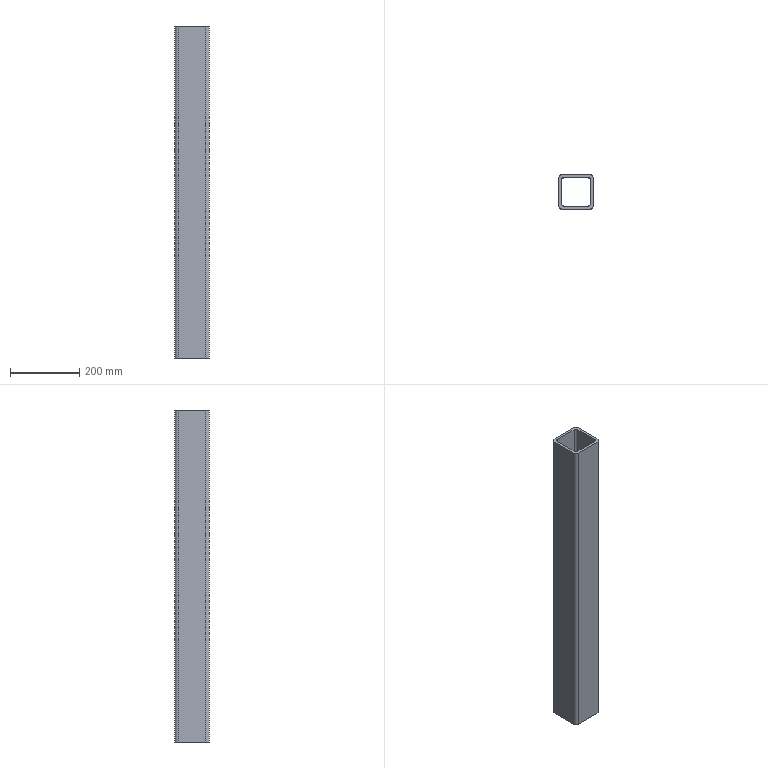Part | SolidWorks | features BaseBody 1 | 1 solid | 18 faces | box 100 x 100 x 960 mm | volume 2796573 mm3 | plane 10 | cylinder 8 | commonest cylinder face diameters 16 x4 20 x4
STEP:
#1=CARTESIAN_POINT('',(10.,96.35,960.));
#2=VERTEX_POINT('',#1);
#3=CARTESIAN_POINT('',(10.,96.35,0.));
#4=VERTEX_POINT('',#3);
#5=CARTESIAN_POINT('',(10.,96.35,960.));
#6=DIRECTION('',(0.,0.,-1.));
#7=VECTOR('',#6,1000.);
#8=LINE('',#5,#7);
#9=EDGE_CURVE('',#2,#4,#8,.T.);
#10=ORIENTED_EDGE('',*,*,#9,.F.);
#11=CARTESIAN_POINT('',(90.,96.35,960.));
#12=VERTEX_POINT('',#11);
#13=CARTESIAN_POINT('',(90.,96.35,960.));
#14=DIRECTION('',(-1.,0.,0.));
#15=VECTOR('',#14,1000.);
#16=LINE('',#13,#15);
#17=EDGE_CURVE('',#12,#2,#16,.T.);
#18=ORIENTED_EDGE('',*,*,#17,.F.);
#19=CARTESIAN_POINT('',(90.,96.35,0.));
#20=VERTEX_POINT('',#19);
#21=CARTESIAN_POINT('',(90.,96.35,960.));
#22=DIRECTION('',(0.,0.,1.));
#23=VECTOR('',#22,1000.);
#24=LINE('',#21,#23);
#25=EDGE_CURVE('',#20,#12,#24,.T.);
#26=ORIENTED_EDGE('',*,*,#25,.F.);
#27=CARTESIAN_POINT('',(90.,96.35,0.));
#28=DIRECTION('',(1.,0.,0.));
#29=VECTOR('',#28,1000.);
#30=LINE('',#27,#29);
#31=EDGE_CURVE('',#4,#20,#30,.T.);
#32=ORIENTED_EDGE('',*,*,#31,.F.);
#33=EDGE_LOOP('',(#10,#18,#26,#32));
#34=FACE_OUTER_BOUND('',#33,.T.);
#35=CARTESIAN_POINT('',(90.,96.35,960.));
#36=DIRECTION('',(0.,-1.,0.));
#37=DIRECTION('',(1.,0.,0.));
#38=AXIS2_PLACEMENT_3D('',#35,#36,#37);
#39=PLANE('',#38);
#40=ADVANCED_FACE('',(#34),#39,.F.);
#41=CARTESIAN_POINT('',(84.,4.35,0.));
#42=VERTEX_POINT('',#41);
#43=CARTESIAN_POINT('',(16.,4.35,0.));
#44=VERTEX_POINT('',#43);
#45=CARTESIAN_POINT('',(10.,4.35,0.));
#46=DIRECTION('',(-1.,0.,0.));
#47=VECTOR('',#46,1000.);
#48=LINE('',#45,#47);
#49=EDGE_CURVE('',#42,#44,#48,.T.);
#50=ORIENTED_EDGE('',*,*,#49,.F.);
#51=CARTESIAN_POINT('',(92.,12.35,0.));
#52=VERTEX_POINT('',#51);
#53=CARTESIAN_POINT('',(84.,12.35,0.));
#54=DIRECTION('',(0.,0.,-1.));
#55=DIRECTION('',(-1.,0.,0.));
#56=AXIS2_PLACEMENT_3D('',#53,#54,#55);
#57=CIRCLE('',#56,8.);
#58=EDGE_CURVE('',#52,#42,#57,.T.);
#59=ORIENTED_EDGE('',*,*,#58,.F.);
#60=CARTESIAN_POINT('',(92.,80.35,0.));
#61=VERTEX_POINT('',#60);
#62=CARTESIAN_POINT('',(92.,86.35,0.));
#63=DIRECTION('',(0.,-1.,0.));
#64=VECTOR('',#63,1000.);
#65=LINE('',#62,#64);
#66=EDGE_CURVE('',#61,#52,#65,.T.);
#67=ORIENTED_EDGE('',*,*,#66,.F.);
#68=CARTESIAN_POINT('',(84.,88.35,0.));
#69=VERTEX_POINT('',#68);
#70=CARTESIAN_POINT('',(84.,80.35,0.));
#71=DIRECTION('',(0.,0.,-1.));
#72=DIRECTION('',(-1.,0.,0.));
#73=AXIS2_PLACEMENT_3D('',#70,#71,#72);
#74=CIRCLE('',#73,8.);
#75=EDGE_CURVE('',#69,#61,#74,.T.);
#76=ORIENTED_EDGE('',*,*,#75,.F.);
#77=CARTESIAN_POINT('',(16.,88.35,0.));
#78=VERTEX_POINT('',#77);
#79=CARTESIAN_POINT('',(10.,88.35,0.));
#80=DIRECTION('',(1.,0.,0.));
#81=VECTOR('',#80,1000.);
#82=LINE('',#79,#81);
#83=EDGE_CURVE('',#78,#69,#82,.T.);
#84=ORIENTED_EDGE('',*,*,#83,.F.);
#85=CARTESIAN_POINT('',(8.,80.35,0.));
#86=VERTEX_POINT('',#85);
#87=CARTESIAN_POINT('',(16.,80.35,0.));
#88=DIRECTION('',(0.,0.,-1.));
#89=DIRECTION('',(-1.,0.,0.));
#90=AXIS2_PLACEMENT_3D('',#87,#88,#89);
#91=CIRCLE('',#90,8.);
#92=EDGE_CURVE('',#86,#78,#91,.T.);
#93=ORIENTED_EDGE('',*,*,#92,.F.);
#94=CARTESIAN_POINT('',(8.,12.35,0.));
#95=VERTEX_POINT('',#94);
#96=CARTESIAN_POINT('',(8.,86.35,0.));
#97=DIRECTION('',(0.,1.,0.));
#98=VECTOR('',#97,1000.);
#99=LINE('',#96,#98);
#100=EDGE_CURVE('',#95,#86,#99,.T.);
#101=ORIENTED_EDGE('',*,*,#100,.F.);
#102=CARTESIAN_POINT('',(16.,12.35,0.));
#103=DIRECTION('',(0.,0.,-1.));
#104=DIRECTION('',(-1.,0.,0.));
#105=AXIS2_PLACEMENT_3D('',#102,#103,#104);
#106=CIRCLE('',#105,8.);
#107=EDGE_CURVE('',#44,#95,#106,.T.);
#108=ORIENTED_EDGE('',*,*,#107,.F.);
#109=EDGE_LOOP('',(#50,#59,#67,#76,#84,#93,#101,#108));
#110=FACE_BOUND('',#109,.T.);
#111=CARTESIAN_POINT('',(100.,86.35,0.));
#112=VERTEX_POINT('',#111);
#113=CARTESIAN_POINT('',(90.,86.35,0.));
#114=DIRECTION('',(0.,0.,1.));
#115=DIRECTION('',(-1.,0.,0.));
#116=AXIS2_PLACEMENT_3D('',#113,#114,#115);
#117=CIRCLE('',#116,10.);
#118=EDGE_CURVE('',#112,#20,#117,.T.);
#119=ORIENTED_EDGE('',*,*,#118,.F.);
#120=CARTESIAN_POINT('',(100.,6.35,0.));
#121=VERTEX_POINT('',#120);
#122=CARTESIAN_POINT('',(100.,86.35,0.));
#123=DIRECTION('',(0.,1.,0.));
#124=VECTOR('',#123,1000.);
#125=LINE('',#122,#124);
#126=EDGE_CURVE('',#121,#112,#125,.T.);
#127=ORIENTED_EDGE('',*,*,#126,.F.);
#128=CARTESIAN_POINT('',(90.,-3.65,0.));
#129=VERTEX_POINT('',#128);
#130=CARTESIAN_POINT('',(90.,6.35,0.));
#131=DIRECTION('',(0.,0.,1.));
#132=DIRECTION('',(-1.,0.,0.));
#133=AXIS2_PLACEMENT_3D('',#130,#131,#132);
#134=CIRCLE('',#133,10.);
#135=EDGE_CURVE('',#129,#121,#134,.T.);
#136=ORIENTED_EDGE('',*,*,#135,.F.);
#137=CARTESIAN_POINT('',(10.,-3.65,0.));
#138=VERTEX_POINT('',#137);
#139=CARTESIAN_POINT('',(10.,-3.65,0.));
#140=DIRECTION('',(1.,0.,0.));
#141=VECTOR('',#140,1000.);
#142=LINE('',#139,#141);
#143=EDGE_CURVE('',#138,#129,#142,.T.);
#144=ORIENTED_EDGE('',*,*,#143,.F.);
#145=CARTESIAN_POINT('',(0.,6.35,0.));
#146=VERTEX_POINT('',#145);
#147=CARTESIAN_POINT('',(10.,6.35,0.));
#148=DIRECTION('',(0.,0.,1.));
#149=DIRECTION('',(-1.,0.,0.));
#150=AXIS2_PLACEMENT_3D('',#147,#148,#149);
#151=CIRCLE('',#150,10.);
#152=EDGE_CURVE('',#146,#138,#151,.T.);
#153=ORIENTED_EDGE('',*,*,#152,.F.);
#154=CARTESIAN_POINT('',(0.,86.35,0.));
#155=VERTEX_POINT('',#154);
#156=CARTESIAN_POINT('',(0.,86.35,0.));
#157=DIRECTION('',(0.,-1.,0.));
#158=VECTOR('',#157,1000.);
#159=LINE('',#156,#158);
#160=EDGE_CURVE('',#155,#146,#159,.T.);
#161=ORIENTED_EDGE('',*,*,#160,.F.);
#162=CARTESIAN_POINT('',(10.,86.35,0.));
#163=DIRECTION('',(0.,0.,1.));
#164=DIRECTION('',(-1.,0.,0.));
#165=AXIS2_PLACEMENT_3D('',#162,#163,#164);
#166=CIRCLE('',#165,10.);
#167=EDGE_CURVE('',#4,#155,#166,.T.);
#168=ORIENTED_EDGE('',*,*,#167,.F.);
#169=ORIENTED_EDGE('',*,*,#31,.T.);
#170=EDGE_LOOP('',(#119,#127,#136,#144,#153,#161,#168,#169));
#171=FACE_OUTER_BOUND('',#170,.T.);
#172=CARTESIAN_POINT('',(10.,86.35,0.));
#173=DIRECTION('',(0.,0.,1.));
#174=DIRECTION('',(1.,0.,0.));
#175=AXIS2_PLACEMENT_3D('',#172,#173,#174);
#176=PLANE('',#175);
#177=ADVANCED_FACE('',(#110,#171),#176,.F.);
#178=CARTESIAN_POINT('',(0.,86.35,960.));
#179=VERTEX_POINT('',#178);
#180=CARTESIAN_POINT('',(10.,86.35,960.));
#181=DIRECTION('',(0.,0.,-1.));
#182=DIRECTION('',(-1.,0.,0.));
#183=AXIS2_PLACEMENT_3D('',#180,#181,#182);
#184=CIRCLE('',#183,10.);
#185=EDGE_CURVE('',#179,#2,#184,.T.);
#186=ORIENTED_EDGE('',*,*,#185,.T.);
#187=ORIENTED_EDGE('',*,*,#9,.T.);
#188=ORIENTED_EDGE('',*,*,#167,.T.);
#189=CARTESIAN_POINT('',(0.,86.35,960.));
#190=DIRECTION('',(0.,0.,1.));
#191=VECTOR('',#190,1000.);
#192=LINE('',#189,#191);
#193=EDGE_CURVE('',#155,#179,#192,.T.);
#194=ORIENTED_EDGE('',*,*,#193,.T.);
#195=EDGE_LOOP('',(#186,#187,#188,#194));
#196=FACE_OUTER_BOUND('',#195,.T.);
#197=CARTESIAN_POINT('',(10.,86.35,960.));
#198=DIRECTION('',(0.,0.,-1.));
#199=DIRECTION('',(-1.,0.,0.));
#200=AXIS2_PLACEMENT_3D('',#197,#198,#199);
#201=CYLINDRICAL_SURFACE('',#200,10.);
#202=ADVANCED_FACE('',(#196),#201,.T.);
#203=CARTESIAN_POINT('',(92.,80.35,960.));
#204=VERTEX_POINT('',#203);
#205=CARTESIAN_POINT('',(92.,12.35,960.));
#206=VERTEX_POINT('',#205);
#207=CARTESIAN_POINT('',(92.,86.35,960.));
#208=DIRECTION('',(0.,-1.,0.));
#209=VECTOR('',#208,1000.);
#210=LINE('',#207,#209);
#211=EDGE_CURVE('',#204,#206,#210,.T.);
#212=ORIENTED_EDGE('',*,*,#211,.T.);
#213=CARTESIAN_POINT('',(84.,4.35,960.));
#214=VERTEX_POINT('',#213);
#215=CARTESIAN_POINT('',(84.,12.35,960.));
#216=DIRECTION('',(0.,0.,-1.));
#217=DIRECTION('',(-1.,0.,0.));
#218=AXIS2_PLACEMENT_3D('',#215,#216,#217);
#219=CIRCLE('',#218,8.);
#220=EDGE_CURVE('',#206,#214,#219,.T.);
#221=ORIENTED_EDGE('',*,*,#220,.T.);
#222=CARTESIAN_POINT('',(16.,4.35,960.));
#223=VERTEX_POINT('',#222);
#224=CARTESIAN_POINT('',(10.,4.35,960.));
#225=DIRECTION('',(-1.,0.,0.));
#226=VECTOR('',#225,1000.);
#227=LINE('',#224,#226);
#228=EDGE_CURVE('',#214,#223,#227,.T.);
#229=ORIENTED_EDGE('',*,*,#228,.T.);
#230=CARTESIAN_POINT('',(8.,12.35,960.));
#231=VERTEX_POINT('',#230);
#232=CARTESIAN_POINT('',(16.,12.35,960.));
#233=DIRECTION('',(0.,0.,-1.));
#234=DIRECTION('',(-1.,0.,0.));
#235=AXIS2_PLACEMENT_3D('',#232,#233,#234);
#236=CIRCLE('',#235,8.);
#237=EDGE_CURVE('',#223,#231,#236,.T.);
#238=ORIENTED_EDGE('',*,*,#237,.T.);
#239=CARTESIAN_POINT('',(8.,80.35,960.));
#240=VERTEX_POINT('',#239);
#241=CARTESIAN_POINT('',(8.,86.35,960.));
#242=DIRECTION('',(0.,1.,0.));
#243=VECTOR('',#242,1000.);
#244=LINE('',#241,#243);
#245=EDGE_CURVE('',#231,#240,#244,.T.);
#246=ORIENTED_EDGE('',*,*,#245,.T.);
#247=CARTESIAN_POINT('',(16.,88.35,960.));
#248=VERTEX_POINT('',#247);
#249=CARTESIAN_POINT('',(16.,80.35,960.));
#250=DIRECTION('',(0.,0.,-1.));
#251=DIRECTION('',(-1.,0.,0.));
#252=AXIS2_PLACEMENT_3D('',#249,#250,#251);
#253=CIRCLE('',#252,8.);
#254=EDGE_CURVE('',#240,#248,#253,.T.);
#255=ORIENTED_EDGE('',*,*,#254,.T.);
#256=CARTESIAN_POINT('',(84.,88.35,960.));
#257=VERTEX_POINT('',#256);
#258=CARTESIAN_POINT('',(10.,88.35,960.));
#259=DIRECTION('',(1.,0.,0.));
#260=VECTOR('',#259,1000.);
#261=LINE('',#258,#260);
#262=EDGE_CURVE('',#248,#257,#261,.T.);
#263=ORIENTED_EDGE('',*,*,#262,.T.);
#264=CARTESIAN_POINT('',(84.,80.35,960.));
#265=DIRECTION('',(0.,0.,-1.));
#266=DIRECTION('',(-1.,0.,0.));
#267=AXIS2_PLACEMENT_3D('',#264,#265,#266);
#268=CIRCLE('',#267,8.);
#269=EDGE_CURVE('',#257,#204,#268,.T.);
#270=ORIENTED_EDGE('',*,*,#269,.T.);
#271=EDGE_LOOP('',(#212,#221,#229,#238,#246,#255,#263,#270));
#272=FACE_BOUND('',#271,.T.);
#273=CARTESIAN_POINT('',(100.,6.35,960.));
#274=VERTEX_POINT('',#273);
#275=CARTESIAN_POINT('',(100.,86.35,960.));
#276=VERTEX_POINT('',#275);
#277=CARTESIAN_POINT('',(100.,86.35,960.));
#278=DIRECTION('',(0.,1.,0.));
#279=VECTOR('',#278,1000.);
#280=LINE('',#277,#279);
#281=EDGE_CURVE('',#274,#276,#280,.T.);
#282=ORIENTED_EDGE('',*,*,#281,.T.);
#283=CARTESIAN_POINT('',(90.,86.35,960.));
#284=DIRECTION('',(0.,0.,1.));
#285=DIRECTION('',(-1.,0.,0.));
#286=AXIS2_PLACEMENT_3D('',#283,#284,#285);
#287=CIRCLE('',#286,10.);
#288=EDGE_CURVE('',#276,#12,#287,.T.);
#289=ORIENTED_EDGE('',*,*,#288,.T.);
#290=ORIENTED_EDGE('',*,*,#17,.T.);
#291=ORIENTED_EDGE('',*,*,#185,.F.);
#292=CARTESIAN_POINT('',(0.,6.35,960.));
#293=VERTEX_POINT('',#292);
#294=CARTESIAN_POINT('',(0.,86.35,960.));
#295=DIRECTION('',(0.,-1.,0.));
#296=VECTOR('',#295,1000.);
#297=LINE('',#294,#296);
#298=EDGE_CURVE('',#179,#293,#297,.T.);
#299=ORIENTED_EDGE('',*,*,#298,.T.);
#300=CARTESIAN_POINT('',(10.,-3.65,960.));
#301=VERTEX_POINT('',#300);
#302=CARTESIAN_POINT('',(10.,6.35,960.));
#303=DIRECTION('',(0.,0.,1.));
#304=DIRECTION('',(-1.,0.,0.));
#305=AXIS2_PLACEMENT_3D('',#302,#303,#304);
#306=CIRCLE('',#305,10.);
#307=EDGE_CURVE('',#293,#301,#306,.T.);
#308=ORIENTED_EDGE('',*,*,#307,.T.);
#309=CARTESIAN_POINT('',(90.,-3.65,960.));
#310=VERTEX_POINT('',#309);
#311=CARTESIAN_POINT('',(10.,-3.65,960.));
#312=DIRECTION('',(1.,0.,0.));
#313=VECTOR('',#312,1000.);
#314=LINE('',#311,#313);
#315=EDGE_CURVE('',#301,#310,#314,.T.);
#316=ORIENTED_EDGE('',*,*,#315,.T.);
#317=CARTESIAN_POINT('',(90.,6.35,960.));
#318=DIRECTION('',(0.,0.,1.));
#319=DIRECTION('',(-1.,0.,0.));
#320=AXIS2_PLACEMENT_3D('',#317,#318,#319);
#321=CIRCLE('',#320,10.);
#322=EDGE_CURVE('',#310,#274,#321,.T.);
#323=ORIENTED_EDGE('',*,*,#322,.T.);
#324=EDGE_LOOP('',(#282,#289,#290,#291,#299,#308,#316,#323));
#325=FACE_OUTER_BOUND('',#324,.T.);
#326=CARTESIAN_POINT('',(10.,86.35,960.));
#327=DIRECTION('',(0.,0.,1.));
#328=DIRECTION('',(1.,0.,0.));
#329=AXIS2_PLACEMENT_3D('',#326,#327,#328);
#330=PLANE('',#329);
#331=ADVANCED_FACE('',(#272,#325),#330,.T.);
#332=ORIENTED_EDGE('',*,*,#288,.F.);
#333=CARTESIAN_POINT('',(100.,86.35,960.));
#334=DIRECTION('',(0.,0.,-1.));
#335=VECTOR('',#334,1000.);
#336=LINE('',#333,#335);
#337=EDGE_CURVE('',#276,#112,#336,.T.);
#338=ORIENTED_EDGE('',*,*,#337,.T.);
#339=ORIENTED_EDGE('',*,*,#118,.T.);
#340=ORIENTED_EDGE('',*,*,#25,.T.);
#341=EDGE_LOOP('',(#332,#338,#339,#340));
#342=FACE_OUTER_BOUND('',#341,.T.);
#343=CARTESIAN_POINT('',(90.,86.35,960.));
#344=DIRECTION('',(0.,0.,-1.));
#345=DIRECTION('',(-1.,0.,0.));
#346=AXIS2_PLACEMENT_3D('',#343,#344,#345);
#347=CYLINDRICAL_SURFACE('',#346,10.);
#348=ADVANCED_FACE('',(#342),#347,.T.);
#349=CARTESIAN_POINT('',(8.,12.35,960.));
#350=DIRECTION('',(0.,0.,-1.));
#351=VECTOR('',#350,1000.);
#352=LINE('',#349,#351);
#353=EDGE_CURVE('',#231,#95,#352,.T.);
#354=ORIENTED_EDGE('',*,*,#353,.F.);
#355=ORIENTED_EDGE('',*,*,#237,.F.);
#356=CARTESIAN_POINT('',(16.,4.35,960.));
#357=DIRECTION('',(0.,0.,1.));
#358=VECTOR('',#357,1000.);
#359=LINE('',#356,#358);
#360=EDGE_CURVE('',#44,#223,#359,.T.);
#361=ORIENTED_EDGE('',*,*,#360,.F.);
#362=ORIENTED_EDGE('',*,*,#107,.T.);
#363=EDGE_LOOP('',(#354,#355,#361,#362));
#364=FACE_OUTER_BOUND('',#363,.T.);
#365=CARTESIAN_POINT('',(16.,12.35,960.));
#366=DIRECTION('',(0.,0.,-1.));
#367=DIRECTION('',(-1.,0.,0.));
#368=AXIS2_PLACEMENT_3D('',#365,#366,#367);
#369=CYLINDRICAL_SURFACE('',#368,8.);
#370=ADVANCED_FACE('',(#364),#369,.F.);
#371=ORIENTED_EDGE('',*,*,#228,.F.);
#372=CARTESIAN_POINT('',(84.,4.35,960.));
#373=DIRECTION('',(0.,0.,-1.));
#374=VECTOR('',#373,1000.);
#375=LINE('',#372,#374);
#376=EDGE_CURVE('',#214,#42,#375,.T.);
#377=ORIENTED_EDGE('',*,*,#376,.T.);
#378=ORIENTED_EDGE('',*,*,#49,.T.);
#379=ORIENTED_EDGE('',*,*,#360,.T.);
#380=EDGE_LOOP('',(#371,#377,#378,#379));
#381=FACE_OUTER_BOUND('',#380,.T.);
#382=CARTESIAN_POINT('',(16.,4.35,960.));
#383=DIRECTION('',(0.,1.,0.));
#384=DIRECTION('',(-1.,0.,0.));
#385=AXIS2_PLACEMENT_3D('',#382,#383,#384);
#386=PLANE('',#385);
#387=ADVANCED_FACE('',(#381),#386,.T.);
#388=ORIENTED_EDGE('',*,*,#376,.F.);
#389=ORIENTED_EDGE('',*,*,#220,.F.);
#390=CARTESIAN_POINT('',(92.,12.35,960.));
#391=DIRECTION('',(0.,0.,1.));
#392=VECTOR('',#391,1000.);
#393=LINE('',#390,#392);
#394=EDGE_CURVE('',#52,#206,#393,.T.);
#395=ORIENTED_EDGE('',*,*,#394,.F.);
#396=ORIENTED_EDGE('',*,*,#58,.T.);
#397=EDGE_LOOP('',(#388,#389,#395,#396));
#398=FACE_OUTER_BOUND('',#397,.T.);
#399=CARTESIAN_POINT('',(84.,12.35,960.));
#400=DIRECTION('',(0.,0.,-1.));
#401=DIRECTION('',(-1.,0.,0.));
#402=AXIS2_PLACEMENT_3D('',#399,#400,#401);
#403=CYLINDRICAL_SURFACE('',#402,8.);
#404=ADVANCED_FACE('',(#398),#403,.F.);
#405=ORIENTED_EDGE('',*,*,#394,.T.);
#406=ORIENTED_EDGE('',*,*,#211,.F.);
#407=CARTESIAN_POINT('',(92.,80.35,960.));
#408=DIRECTION('',(0.,0.,1.));
#409=VECTOR('',#408,1000.);
#410=LINE('',#407,#409);
#411=EDGE_CURVE('',#61,#204,#410,.T.);
#412=ORIENTED_EDGE('',*,*,#411,.F.);
#413=ORIENTED_EDGE('',*,*,#66,.T.);
#414=EDGE_LOOP('',(#405,#406,#412,#413));
#415=FACE_OUTER_BOUND('',#414,.T.);
#416=CARTESIAN_POINT('',(92.,80.35,960.));
#417=DIRECTION('',(1.,0.,0.));
#418=DIRECTION('',(0.,1.,0.));
#419=AXIS2_PLACEMENT_3D('',#416,#417,#418);
#420=PLANE('',#419);
#421=ADVANCED_FACE('',(#415),#420,.F.);
#422=ORIENTED_EDGE('',*,*,#411,.T.);
#423=ORIENTED_EDGE('',*,*,#269,.F.);
#424=CARTESIAN_POINT('',(84.,88.35,960.));
#425=DIRECTION('',(0.,0.,1.));
#426=VECTOR('',#425,1000.);
#427=LINE('',#424,#426);
#428=EDGE_CURVE('',#69,#257,#427,.T.);
#429=ORIENTED_EDGE('',*,*,#428,.F.);
#430=ORIENTED_EDGE('',*,*,#75,.T.);
#431=EDGE_LOOP('',(#422,#423,#429,#430));
#432=FACE_OUTER_BOUND('',#431,.T.);
#433=CARTESIAN_POINT('',(84.,80.35,960.));
#434=DIRECTION('',(0.,0.,-1.));
#435=DIRECTION('',(-1.,0.,0.));
#436=AXIS2_PLACEMENT_3D('',#433,#434,#435);
#437=CYLINDRICAL_SURFACE('',#436,8.);
#438=ADVANCED_FACE('',(#432),#437,.F.);
#439=ORIENTED_EDGE('',*,*,#262,.F.);
#440=CARTESIAN_POINT('',(16.,88.35,960.));
#441=DIRECTION('',(0.,0.,-1.));
#442=VECTOR('',#441,1000.);
#443=LINE('',#440,#442);
#444=EDGE_CURVE('',#248,#78,#443,.T.);
#445=ORIENTED_EDGE('',*,*,#444,.T.);
#446=ORIENTED_EDGE('',*,*,#83,.T.);
#447=ORIENTED_EDGE('',*,*,#428,.T.);
#448=EDGE_LOOP('',(#439,#445,#446,#447));
#449=FACE_OUTER_BOUND('',#448,.T.);
#450=CARTESIAN_POINT('',(84.,88.35,960.));
#451=DIRECTION('',(0.,-1.,0.));
#452=DIRECTION('',(1.,0.,0.));
#453=AXIS2_PLACEMENT_3D('',#450,#451,#452);
#454=PLANE('',#453);
#455=ADVANCED_FACE('',(#449),#454,.T.);
#456=ORIENTED_EDGE('',*,*,#444,.F.);
#457=ORIENTED_EDGE('',*,*,#254,.F.);
#458=CARTESIAN_POINT('',(8.,80.35,960.));
#459=DIRECTION('',(0.,0.,1.));
#460=VECTOR('',#459,1000.);
#461=LINE('',#458,#460);
#462=EDGE_CURVE('',#86,#240,#461,.T.);
#463=ORIENTED_EDGE('',*,*,#462,.F.);
#464=ORIENTED_EDGE('',*,*,#92,.T.);
#465=EDGE_LOOP('',(#456,#457,#463,#464));
#466=FACE_OUTER_BOUND('',#465,.T.);
#467=CARTESIAN_POINT('',(16.,80.35,960.));
#468=DIRECTION('',(0.,0.,-1.));
#469=DIRECTION('',(-1.,0.,0.));
#470=AXIS2_PLACEMENT_3D('',#467,#468,#469);
#471=CYLINDRICAL_SURFACE('',#470,8.);
#472=ADVANCED_FACE('',(#466),#471,.F.);
#473=ORIENTED_EDGE('',*,*,#462,.T.);
#474=ORIENTED_EDGE('',*,*,#245,.F.);
#475=ORIENTED_EDGE('',*,*,#353,.T.);
#476=ORIENTED_EDGE('',*,*,#100,.T.);
#477=EDGE_LOOP('',(#473,#474,#475,#476));
#478=FACE_OUTER_BOUND('',#477,.T.);
#479=CARTESIAN_POINT('',(8.,12.35,960.));
#480=DIRECTION('',(-1.,0.,0.));
#481=DIRECTION('',(0.,-1.,0.));
#482=AXIS2_PLACEMENT_3D('',#479,#480,#481);
#483=PLANE('',#482);
#484=ADVANCED_FACE('',(#478),#483,.F.);
#485=ORIENTED_EDGE('',*,*,#281,.F.);
#486=CARTESIAN_POINT('',(100.,6.35,960.));
#487=DIRECTION('',(0.,0.,-1.));
#488=VECTOR('',#487,1000.);
#489=LINE('',#486,#488);
#490=EDGE_CURVE('',#274,#121,#489,.T.);
#491=ORIENTED_EDGE('',*,*,#490,.T.);
#492=ORIENTED_EDGE('',*,*,#126,.T.);
#493=ORIENTED_EDGE('',*,*,#337,.F.);
#494=EDGE_LOOP('',(#485,#491,#492,#493));
#495=FACE_OUTER_BOUND('',#494,.T.);
#496=CARTESIAN_POINT('',(100.,86.35,960.));
#497=DIRECTION('',(1.,0.,0.));
#498=DIRECTION('',(0.,0.,-1.));
#499=AXIS2_PLACEMENT_3D('',#496,#497,#498);
#500=PLANE('',#499);
#501=ADVANCED_FACE('',(#495),#500,.T.);
#502=ORIENTED_EDGE('',*,*,#322,.F.);
#503=CARTESIAN_POINT('',(90.,-3.65,960.));
#504=DIRECTION('',(0.,0.,-1.));
#505=VECTOR('',#504,1000.);
#506=LINE('',#503,#505);
#507=EDGE_CURVE('',#310,#129,#506,.T.);
#508=ORIENTED_EDGE('',*,*,#507,.T.);
#509=ORIENTED_EDGE('',*,*,#135,.T.);
#510=ORIENTED_EDGE('',*,*,#490,.F.);
#511=EDGE_LOOP('',(#502,#508,#509,#510));
#512=FACE_OUTER_BOUND('',#511,.T.);
#513=CARTESIAN_POINT('',(90.,6.35,960.));
#514=DIRECTION('',(0.,0.,-1.));
#515=DIRECTION('',(-1.,0.,0.));
#516=AXIS2_PLACEMENT_3D('',#513,#514,#515);
#517=CYLINDRICAL_SURFACE('',#516,10.);
#518=ADVANCED_FACE('',(#512),#517,.T.);
#519=ORIENTED_EDGE('',*,*,#507,.F.);
#520=ORIENTED_EDGE('',*,*,#315,.F.);
#521=CARTESIAN_POINT('',(10.,-3.65,960.));
#522=DIRECTION('',(0.,0.,1.));
#523=VECTOR('',#522,1000.);
#524=LINE('',#521,#523);
#525=EDGE_CURVE('',#138,#301,#524,.T.);
#526=ORIENTED_EDGE('',*,*,#525,.F.);
#527=ORIENTED_EDGE('',*,*,#143,.T.);
#528=EDGE_LOOP('',(#519,#520,#526,#527));
#529=FACE_OUTER_BOUND('',#528,.T.);
#530=CARTESIAN_POINT('',(10.,-3.65,960.));
#531=DIRECTION('',(0.,1.,0.));
#532=DIRECTION('',(-1.,0.,0.));
#533=AXIS2_PLACEMENT_3D('',#530,#531,#532);
#534=PLANE('',#533);
#535=ADVANCED_FACE('',(#529),#534,.F.);
#536=ORIENTED_EDGE('',*,*,#307,.F.);
#537=CARTESIAN_POINT('',(0.,6.35,960.));
#538=DIRECTION('',(0.,0.,-1.));
#539=VECTOR('',#538,1000.);
#540=LINE('',#537,#539);
#541=EDGE_CURVE('',#293,#146,#540,.T.);
#542=ORIENTED_EDGE('',*,*,#541,.T.);
#543=ORIENTED_EDGE('',*,*,#152,.T.);
#544=ORIENTED_EDGE('',*,*,#525,.T.);
#545=EDGE_LOOP('',(#536,#542,#543,#544));
#546=FACE_OUTER_BOUND('',#545,.T.);
#547=CARTESIAN_POINT('',(10.,6.35,960.));
#548=DIRECTION('',(0.,0.,-1.));
#549=DIRECTION('',(-1.,0.,0.));
#550=AXIS2_PLACEMENT_3D('',#547,#548,#549);
#551=CYLINDRICAL_SURFACE('',#550,10.);
#552=ADVANCED_FACE('',(#546),#551,.T.);
#553=ORIENTED_EDGE('',*,*,#298,.F.);
#554=ORIENTED_EDGE('',*,*,#193,.F.);
#555=ORIENTED_EDGE('',*,*,#160,.T.);
#556=ORIENTED_EDGE('',*,*,#541,.F.);
#557=EDGE_LOOP('',(#553,#554,#555,#556));
#558=FACE_OUTER_BOUND('',#557,.T.);
#559=CARTESIAN_POINT('',(0.,6.35,960.));
#560=DIRECTION('',(-1.,0.,0.));
#561=DIRECTION('',(0.,-1.,0.));
#562=AXIS2_PLACEMENT_3D('',#559,#560,#561);
#563=PLANE('',#562);
#564=ADVANCED_FACE('',(#558),#563,.T.);
#565=CLOSED_SHELL('',(#40,#177,#202,#331,#348,#370,#387,#404,#421,#438,#455,#472,#484,#501,#518,#535,#552,#564));
#566=MANIFOLD_SOLID_BREP('',#565);
#567=CARTESIAN_POINT('',(0.,0.,0.));
#568=DIRECTION('',(0.,0.,1.));
#569=DIRECTION('',(1.,0.,0.));
#570=AXIS2_PLACEMENT_3D('',#567,#568,#569);
#571=(LENGTH_UNIT()NAMED_UNIT(*)SI_UNIT(.MILLI.,.METRE.));
#572=UNCERTAINTY_MEASURE_WITH_UNIT(LENGTH_MEASURE(0.00001),#571,'','');
#573=(NAMED_UNIT(*)PLANE_ANGLE_UNIT()SI_UNIT($,.RADIAN.));
#574=(NAMED_UNIT(*)SI_UNIT($,.STERADIAN.)SOLID_ANGLE_UNIT());
#575=(GEOMETRIC_REPRESENTATION_CONTEXT(3)GLOBAL_UNCERTAINTY_ASSIGNED_CONTEXT((#572))GLOBAL_UNIT_ASSIGNED_CONTEXT((#571,#573,#574))REPRESENTATION_CONTEXT('',''));
#576=ADVANCED_BREP_SHAPE_REPRESENTATION('',(#566,#570),#575);